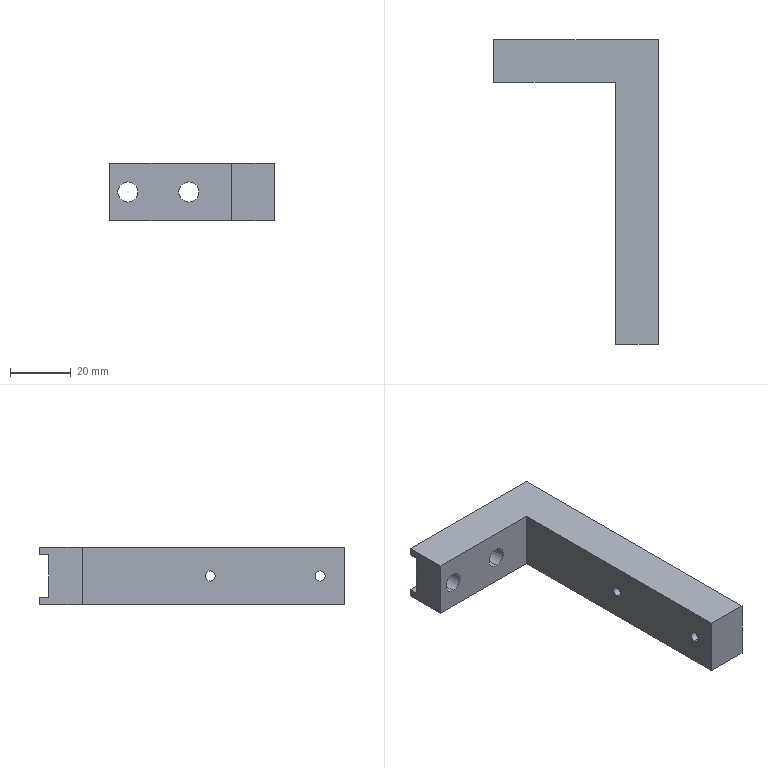Part | STEP file | PN_0063 gripper jaw | 1 solid | 20 faces | box 54 x 100 x 19 mm | volume 33980 mm3 | plane 12 | cylinder 8 | commonest cylinder face diameters 3.3 x4 6.6 x4